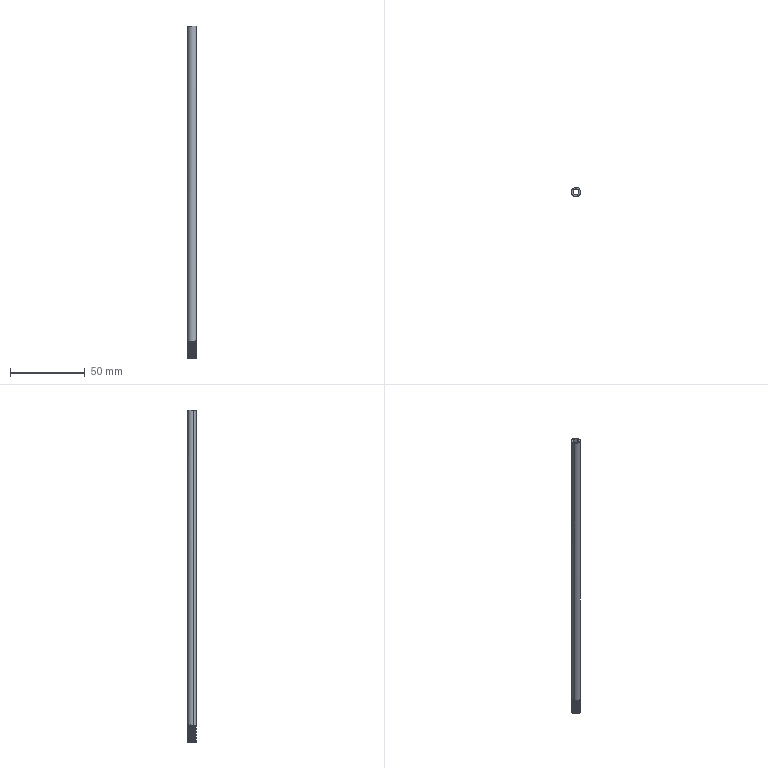Part | SolidWorks | features BaseBody 1 | 1 solid | 57 faces | box 6 x 6 x 222.5 mm | volume 3441 mm3 | cylinder 49 | plane 4 | cone 2 | spline 2 | commonest cylinder face diameters 6 x24 5 x23 4 x2